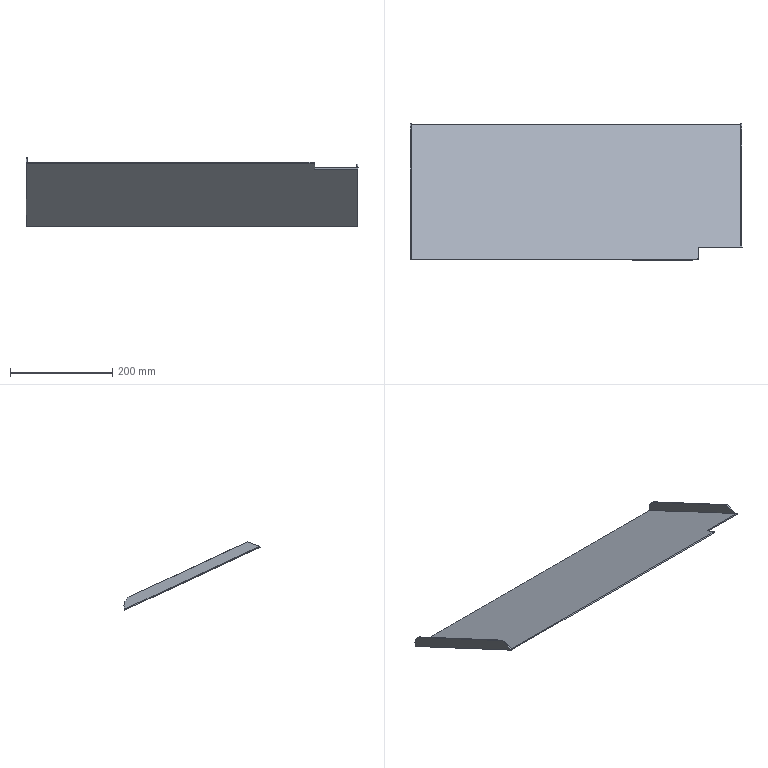Part | NX | features solid 2 | 1 solid | 21 faces | box 650 x 266.54 x 133.86 mm | volume 390473 mm3 | plane 15 | spline 4 | cylinder 2 | commonest cylinder face diameters 40 x2
STEP:
#1=CARTESIAN_POINT('',(363.,820.,-235.638));
#2=VERTEX_POINT('',#1);
#3=CARTESIAN_POINT('',(363.,820.,-233.432));
#4=VERTEX_POINT('',#3);
#5=CARTESIAN_POINT('',(363.,820.,-700.));
#6=DIRECTION('',(0.,0.,-1.));
#7=VECTOR('',#6,1000.);
#8=LINE('',#5,#7);
#9=EDGE_CURVE('',#2,#4,#8,.F.);
#10=ORIENTED_EDGE('',*,*,#9,.F.);
#11=CARTESIAN_POINT('',(280.,820.,-235.638));
#12=VERTEX_POINT('',#11);
#13=CARTESIAN_POINT('',(280.,820.,-235.638));
#14=CARTESIAN_POINT('',(307.667,820.,-235.638));
#15=CARTESIAN_POINT('',(335.333,820.,-235.638));
#16=CARTESIAN_POINT('',(363.,820.,-235.638));
#17=B_SPLINE_CURVE_WITH_KNOTS('',3,(#13,#14,#15,#16),.UNSPECIFIED.,.F.,.F.,(4,4),(0.,0.9765),.UNSPECIFIED.);
#18=EDGE_CURVE('',#12,#2,#17,.T.);
#19=ORIENTED_EDGE('',*,*,#18,.F.);
#20=CARTESIAN_POINT('',(-283.,820.,-235.638));
#21=VERTEX_POINT('',#20);
#22=CARTESIAN_POINT('',(1065.,820.,-235.638));
#23=DIRECTION('',(-1.,0.,0.));
#24=VECTOR('',#23,1000.);
#25=LINE('',#22,#24);
#26=EDGE_CURVE('',#21,#12,#25,.F.);
#27=ORIENTED_EDGE('',*,*,#26,.F.);
#28=CARTESIAN_POINT('',(-283.,820.,-233.432));
#29=VERTEX_POINT('',#28);
#30=CARTESIAN_POINT('',(-283.,820.,-700.));
#31=DIRECTION('',(0.,0.,1.));
#32=VECTOR('',#31,1000.);
#33=LINE('',#30,#32);
#34=EDGE_CURVE('',#29,#21,#33,.F.);
#35=ORIENTED_EDGE('',*,*,#34,.F.);
#36=CARTESIAN_POINT('',(1065.,820.,-233.432));
#37=DIRECTION('',(-1.,0.,0.));
#38=VECTOR('',#37,1000.);
#39=LINE('',#36,#38);
#40=EDGE_CURVE('',#29,#4,#39,.F.);
#41=ORIENTED_EDGE('',*,*,#40,.T.);
#42=EDGE_LOOP('',(#10,#19,#27,#35,#41));
#43=FACE_BOUND('',#42,.T.);
#44=CARTESIAN_POINT('',(1065.,820.,-700.));
#45=DIRECTION('',(0.,-1.,0.));
#46=DIRECTION('',(-1.,0.,0.));
#47=AXIS2_PLACEMENT_3D('',#44,#45,#46);
#48=PLANE('',#47);
#49=ADVANCED_FACE('',(#43),#48,.F.);
#50=CARTESIAN_POINT('',(363.,582.799,-122.823));
#51=VERTEX_POINT('',#50);
#52=CARTESIAN_POINT('',(363.,569.539,-116.64));
#53=DIRECTION('',(0.,-0.9063,0.4226));
#54=VECTOR('',#53,1000.);
#55=LINE('',#52,#54);
#56=EDGE_CURVE('',#4,#51,#55,.T.);
#57=ORIENTED_EDGE('',*,*,#56,.F.);
#58=ORIENTED_EDGE('',*,*,#40,.F.);
#59=CARTESIAN_POINT('',(-283.,556.355,-110.492));
#60=VERTEX_POINT('',#59);
#61=CARTESIAN_POINT('',(-283.,569.539,-116.64));
#62=DIRECTION('',(0.,0.9063,-0.4226));
#63=VECTOR('',#62,1000.);
#64=LINE('',#61,#63);
#65=EDGE_CURVE('',#60,#29,#64,.T.);
#66=ORIENTED_EDGE('',*,*,#65,.F.);
#67=CARTESIAN_POINT('',(280.,557.997,-111.258));
#68=VERTEX_POINT('',#67);
#69=CARTESIAN_POINT('',(-283.,556.355,-110.492));
#70=CARTESIAN_POINT('',(-278.931,556.386,-110.507));
#71=CARTESIAN_POINT('',(-273.683,556.424,-110.524));
#72=CARTESIAN_POINT('',(-269.093,556.45,-110.536));
#73=CARTESIAN_POINT('',(-266.871,556.46,-110.541));
#74=CARTESIAN_POINT('',(-265.734,556.464,-110.543));
#75=CARTESIAN_POINT('',(-264.768,556.467,-110.544));
#76=CARTESIAN_POINT('',(-264.472,556.467,-110.544));
#77=CARTESIAN_POINT('',(-263.335,556.469,-110.545));
#78=CARTESIAN_POINT('',(-260.973,556.47,-110.546));
#79=CARTESIAN_POINT('',(-257.355,556.471,-110.546));
#80=CARTESIAN_POINT('',(-253.755,556.471,-110.546));
#81=CARTESIAN_POINT('',(-251.203,556.471,-110.546));
#82=CARTESIAN_POINT('',(-248.985,556.47,-110.546));
#83=CARTESIAN_POINT('',(-247.518,556.47,-110.546));
#84=CARTESIAN_POINT('',(-246.313,556.47,-110.546));
#85=CARTESIAN_POINT('',(-245.51,556.47,-110.546));
#86=CARTESIAN_POINT('',(-245.,556.47,-110.546));
#87=CARTESIAN_POINT('',(-244.61,556.47,-110.546));
#88=CARTESIAN_POINT('',(-244.577,556.47,-110.546));
#89=CARTESIAN_POINT('',(-244.438,556.47,-110.546));
#90=CARTESIAN_POINT('',(-244.266,556.47,-110.546));
#91=CARTESIAN_POINT('',(-244.029,556.47,-110.546));
#92=CARTESIAN_POINT('',(-243.648,556.47,-110.546));
#93=CARTESIAN_POINT('',(-243.15,556.47,-110.546));
#94=CARTESIAN_POINT('',(-242.522,556.47,-110.546));
#95=CARTESIAN_POINT('',(-241.644,556.47,-110.546));
#96=CARTESIAN_POINT('',(-240.468,556.47,-110.546));
#97=CARTESIAN_POINT('',(-238.932,556.47,-110.546));
#98=CARTESIAN_POINT('',(-237.272,556.47,-110.546));
#99=CARTESIAN_POINT('',(-234.893,556.471,-110.546));
#100=CARTESIAN_POINT('',(-231.608,556.471,-110.546));
#101=CARTESIAN_POINT('',(-227.169,556.472,-110.547));
#102=CARTESIAN_POINT('',(-222.234,556.474,-110.547));
#103=CARTESIAN_POINT('',(-217.705,556.475,-110.548));
#104=CARTESIAN_POINT('',(-213.835,556.477,-110.549));
#105=CARTESIAN_POINT('',(-210.805,556.478,-110.549));
#106=CARTESIAN_POINT('',(-208.187,556.479,-110.55));
#107=CARTESIAN_POINT('',(-206.278,556.479,-110.55));
#108=CARTESIAN_POINT('',(-205.207,556.48,-110.55));
#109=CARTESIAN_POINT('',(-204.295,556.48,-110.55));
#110=CARTESIAN_POINT('',(-203.762,556.48,-110.55));
#111=CARTESIAN_POINT('',(-202.967,556.48,-110.551));
#112=CARTESIAN_POINT('',(-201.617,556.481,-110.551));
#113=CARTESIAN_POINT('',(-199.674,556.482,-110.551));
#114=CARTESIAN_POINT('',(-197.361,556.482,-110.551));
#115=CARTESIAN_POINT('',(-194.288,556.484,-110.552));
#116=CARTESIAN_POINT('',(-190.473,556.485,-110.553));
#117=CARTESIAN_POINT('',(-184.421,556.487,-110.553));
#118=CARTESIAN_POINT('',(-176.957,556.489,-110.554));
#119=CARTESIAN_POINT('',(-168.157,556.491,-110.555));
#120=CARTESIAN_POINT('',(-159.529,556.493,-110.556));
#121=CARTESIAN_POINT('',(-151.02,556.494,-110.557));
#122=CARTESIAN_POINT('',(-144.193,556.495,-110.557));
#123=CARTESIAN_POINT('',(-138.373,556.496,-110.558));
#124=CARTESIAN_POINT('',(-132.608,556.496,-110.558));
#125=CARTESIAN_POINT('',(-122.474,556.497,-110.558));
#126=CARTESIAN_POINT('',(-107.961,556.497,-110.558));
#127=CARTESIAN_POINT('',(-90.461,556.496,-110.558));
#128=CARTESIAN_POINT('',(-67.026,556.492,-110.556));
#129=CARTESIAN_POINT('',(-43.429,556.486,-110.553));
#130=CARTESIAN_POINT('',(-22.654,556.478,-110.549));
#131=CARTESIAN_POINT('',(-10.728,556.473,-110.547));
#132=CARTESIAN_POINT('',(-1.807,556.469,-110.545));
#133=CARTESIAN_POINT('',(7.39,556.464,-110.543));
#134=CARTESIAN_POINT('',(19.483,556.458,-110.54));
#135=CARTESIAN_POINT('',(40.546,556.446,-110.534));
#136=CARTESIAN_POINT('',(64.247,556.429,-110.527));
#137=CARTESIAN_POINT('',(87.609,556.411,-110.518));
#138=CARTESIAN_POINT('',(104.953,556.395,-110.511));
#139=CARTESIAN_POINT('',(119.271,556.382,-110.504));
#140=CARTESIAN_POINT('',(129.2,556.372,-110.5));
#141=CARTESIAN_POINT('',(134.878,556.366,-110.497));
#142=CARTESIAN_POINT('',(139.051,556.361,-110.495));
#143=CARTESIAN_POINT('',(143.632,556.356,-110.493));
#144=CARTESIAN_POINT('',(149.578,556.35,-110.49));
#145=CARTESIAN_POINT('',(160.009,556.338,-110.484));
#146=CARTESIAN_POINT('',(174.758,556.32,-110.476));
#147=CARTESIAN_POINT('',(189.34,556.301,-110.467));
#148=CARTESIAN_POINT('',(200.949,556.285,-110.459));
#149=CARTESIAN_POINT('',(209.492,556.273,-110.454));
#150=CARTESIAN_POINT('',(218.464,556.26,-110.448));
#151=CARTESIAN_POINT('',(227.262,556.247,-110.441));
#152=CARTESIAN_POINT('',(236.065,556.233,-110.435));
#153=CARTESIAN_POINT('',(244.756,556.219,-110.428));
#154=CARTESIAN_POINT('',(252.156,556.206,-110.423));
#155=CARTESIAN_POINT('',(257.28,556.198,-110.419));
#156=CARTESIAN_POINT('',(260.209,556.193,-110.416));
#157=CARTESIAN_POINT('',(262.031,556.189,-110.415));
#158=CARTESIAN_POINT('',(263.502,556.187,-110.414));
#159=CARTESIAN_POINT('',(264.602,556.185,-110.413));
#160=CARTESIAN_POINT('',(265.522,556.183,-110.412));
#161=CARTESIAN_POINT('',(266.158,556.182,-110.411));
#162=CARTESIAN_POINT('',(266.534,556.182,-110.411));
#163=CARTESIAN_POINT('',(266.779,556.181,-110.411));
#164=CARTESIAN_POINT('',(267.335,556.18,-110.411));
#165=CARTESIAN_POINT('',(267.867,556.18,-110.41));
#166=CARTESIAN_POINT('',(268.429,556.179,-110.41));
#167=CARTESIAN_POINT('',(268.765,556.179,-110.41));
#168=CARTESIAN_POINT('',(268.942,556.181,-110.411));
#169=CARTESIAN_POINT('',(268.947,556.18,-110.41));
#170=CARTESIAN_POINT('',(269.298,556.193,-110.417));
#171=CARTESIAN_POINT('',(269.627,556.217,-110.428));
#172=CARTESIAN_POINT('',(270.088,556.271,-110.453));
#173=CARTESIAN_POINT('',(270.202,556.291,-110.462));
#174=CARTESIAN_POINT('',(270.458,556.333,-110.482));
#175=CARTESIAN_POINT('',(270.765,556.386,-110.506));
#176=CARTESIAN_POINT('',(271.258,556.471,-110.546));
#177=CARTESIAN_POINT('',(271.394,556.495,-110.557));
#178=CARTESIAN_POINT('',(271.708,556.55,-110.583));
#179=CARTESIAN_POINT('',(272.066,556.613,-110.612));
#180=CARTESIAN_POINT('',(272.531,556.694,-110.65));
#181=CARTESIAN_POINT('',(273.483,556.86,-110.728));
#182=CARTESIAN_POINT('',(275.728,557.252,-110.91));
#183=CARTESIAN_POINT('',(278.187,557.681,-111.11));
#184=CARTESIAN_POINT('',(280.,557.997,-111.258));
#185=B_SPLINE_CURVE_WITH_KNOTS('',3,(#69,#70,#71,#72,#73,#74,#75,#76,#77,#78,#79,#80,#81,#82,#83,#84,#85,#86,#87,#88,#89,#90,#91,#92,#93,#94,#95,#96,#97,#98,#99,#100,#101,#102,#103,#104,#105,#106,#107,#108,#109,#110,#111,#112,#113,#114,#115,#116,#117,#118,#119,#120,#121,#122,#123,#124,#125,#126,#127,#128,#129,#130,#131,#132,#133,#134,#135,#136,#137,#138,#139,#140,#141,#142,#143,#144,#145,#146,#147,#148,#149,#150,#151,#152,#153,#154,#155,#156,#157,#158,#159,#160,#161,#162,#163,#164,#165,#166,#167,#168,#169,#170,#171,#172,#173,#174,#175,#176,#177,#178,#179,#180,#181,#182,#183,#184),.UNSPECIFIED.,.F.,.F.,(4,1,1,1,1,1,1,1,1,1,1,1,1,1,1,1,1,1,1,1,1,1,1,1,1,1,1,1,1,1,1,1,1,1,1,1,1,1,1,1,1,1,1,1,1,1,1,1,1,1,1,1,1,1,1,1,1,1,1,1,1,1,1,1,1,1,1,1,1,1,1,1,1,1,1,1,1,1,1,1,1,1,1,1,1,1,1,1,1,1,1,1,1,1,1,1,1,1,1,1,1,1,1,1,1,1,1,1,1,1,1,1,1,4),(0.002497,0.01808,0.02588,0.02977,0.03367,0.03562,0.03757,0.04146,0.04925,0.05705,0.06094,0.06484,0.06679,0.06874,0.06971,0.07069,0.07117,0.07142,0.07166,0.07215,0.07263,0.07361,0.07458,0.07653,0.07848,0.08043,0.08432,0.08822,0.09212,0.09601,0.1038,0.1116,0.1194,0.1272,0.1311,0.135,0.1389,0.1408,0.1418,0.1428,0.1437,0.1447,0.1467,0.1506,0.1545,0.1584,0.1661,0.1739,0.1895,0.2051,0.2207,0.2363,0.2519,0.2597,0.2675,0.283,0.3142,0.3454,0.3766,0.4389,0.4701,0.4857,0.5012,0.5168,0.5324,0.5636,0.6259,0.6571,0.6883,0.7195,0.735,0.7428,0.7506,0.7584,0.7662,0.7818,0.813,0.8441,0.8597,0.8753,0.8909,0.9065,0.9221,0.9377,0.9532,0.961,0.9649,0.9688,0.9708,0.9727,0.9747,0.9756,0.9761,0.9766,0.9771,0.9776,0.9786,0.9795,0.98,0.9805,0.981,0.9815,0.9825,0.983,0.9834,0.9839,0.9844,0.9849,0.9854,0.9864,0.9873,0.9883,0.9922,1.),.UNSPECIFIED.);
#186=EDGE_CURVE('',#60,#68,#185,.T.);
#187=ORIENTED_EDGE('',*,*,#186,.T.);
#188=CARTESIAN_POINT('',(280.,580.313,-121.664));
#189=VERTEX_POINT('',#188);
#190=CARTESIAN_POINT('',(280.,569.539,-116.64));
#191=DIRECTION('',(0.,0.9063,-0.4226));
#192=VECTOR('',#191,1000.);
#193=LINE('',#190,#192);
#194=EDGE_CURVE('',#68,#189,#193,.T.);
#195=ORIENTED_EDGE('',*,*,#194,.T.);
#196=CARTESIAN_POINT('',(365.,580.142,-121.584));
#197=VERTEX_POINT('',#196);
#198=CARTESIAN_POINT('',(280.,580.313,-121.664));
#199=CARTESIAN_POINT('',(308.333,580.262,-121.64));
#200=CARTESIAN_POINT('',(336.667,580.205,-121.614));
#201=CARTESIAN_POINT('',(365.,580.142,-121.584));
#202=B_SPLINE_CURVE_WITH_KNOTS('',3,(#198,#199,#200,#201),.UNSPECIFIED.,.F.,.F.,(4,4),(0.,0.085),.UNSPECIFIED.);
#203=EDGE_CURVE('',#189,#197,#202,.T.);
#204=ORIENTED_EDGE('',*,*,#203,.T.);
#205=CARTESIAN_POINT('',(365.,582.799,-122.823));
#206=VERTEX_POINT('',#205);
#207=CARTESIAN_POINT('',(365.,569.539,-116.64));
#208=DIRECTION('',(0.,0.9063,-0.4226));
#209=VECTOR('',#208,1000.);
#210=LINE('',#207,#209);
#211=EDGE_CURVE('',#197,#206,#210,.T.);
#212=ORIENTED_EDGE('',*,*,#211,.T.);
#213=CARTESIAN_POINT('',(-285.,582.799,-122.823));
#214=DIRECTION('',(-1.,0.,0.));
#215=VECTOR('',#214,1000.);
#216=LINE('',#213,#215);
#217=EDGE_CURVE('',#51,#206,#216,.F.);
#218=ORIENTED_EDGE('',*,*,#217,.F.);
#219=EDGE_LOOP('',(#57,#58,#66,#187,#195,#204,#212,#218));
#220=FACE_BOUND('',#219,.T.);
#221=CARTESIAN_POINT('',(-285.,569.539,-116.64));
#222=DIRECTION('',(0.,0.4226,0.9063));
#223=DIRECTION('',(1.,0.,0.));
#224=AXIS2_PLACEMENT_3D('',#221,#222,#223);
#225=PLANE('',#224);
#226=ADVANCED_FACE('',(#220),#225,.T.);
#227=CARTESIAN_POINT('',(-285.,810.326,-209.06));
#228=VERTEX_POINT('',#227);
#229=CARTESIAN_POINT('',(-285.,820.,-235.638));
#230=VERTEX_POINT('',#229);
#231=CARTESIAN_POINT('',(-285.,801.874,-227.186));
#232=DIRECTION('',(1.,0.,0.));
#233=DIRECTION('',(0.,1.,0.));
#234=AXIS2_PLACEMENT_3D('',#231,#232,#233);
#235=CIRCLE('',#234,20.);
#236=EDGE_CURVE('',#228,#230,#235,.F.);
#237=ORIENTED_EDGE('',*,*,#236,.T.);
#238=CARTESIAN_POINT('',(-285.,555.494,-112.297));
#239=VERTEX_POINT('',#238);
#240=CARTESIAN_POINT('',(-285.,568.694,-118.452));
#241=DIRECTION('',(0.,0.9063,-0.4226));
#242=VECTOR('',#241,1000.);
#243=LINE('',#240,#242);
#244=EDGE_CURVE('',#239,#230,#243,.T.);
#245=ORIENTED_EDGE('',*,*,#244,.F.);
#246=CARTESIAN_POINT('',(-285.,556.339,-110.485));
#247=VERTEX_POINT('',#246);
#248=CARTESIAN_POINT('',(-285.,555.494,-112.297));
#249=DIRECTION('',(0.,0.4226,0.9063));
#250=VECTOR('',#249,1000.);
#251=LINE('',#248,#250);
#252=EDGE_CURVE('',#239,#247,#251,.T.);
#253=ORIENTED_EDGE('',*,*,#252,.T.);
#254=CARTESIAN_POINT('',(-285.,580.26,-101.778));
#255=VERTEX_POINT('',#254);
#256=CARTESIAN_POINT('',(-285.,580.26,-101.778));
#257=DIRECTION('',(0.,-0.9397,-0.342));
#258=VECTOR('',#257,1000.);
#259=LINE('',#256,#258);
#260=EDGE_CURVE('',#247,#255,#259,.F.);
#261=ORIENTED_EDGE('',*,*,#260,.T.);
#262=CARTESIAN_POINT('',(-285.,563.946,-94.171));
#263=DIRECTION('',(0.,0.9063,-0.4226));
#264=VECTOR('',#263,1000.);
#265=LINE('',#262,#264);
#266=EDGE_CURVE('',#255,#228,#265,.T.);
#267=ORIENTED_EDGE('',*,*,#266,.T.);
#268=EDGE_LOOP('',(#237,#245,#253,#261,#267));
#269=FACE_BOUND('',#268,.T.);
#270=CARTESIAN_POINT('',(-285.,569.539,-116.64));
#271=DIRECTION('',(-1.,0.,0.));
#272=DIRECTION('',(0.,-1.,0.));
#273=AXIS2_PLACEMENT_3D('',#270,#271,#272);
#274=PLANE('',#273);
#275=ADVANCED_FACE('',(#269),#274,.T.);
#276=ORIENTED_EDGE('',*,*,#186,.F.);
#277=CARTESIAN_POINT('',(-283.,555.502,-112.301));
#278=VERTEX_POINT('',#277);
#279=CARTESIAN_POINT('',(-283.,556.355,-110.492));
#280=DIRECTION('',(0.,-0.4226,-0.9063));
#281=VECTOR('',#280,1000.);
#282=LINE('',#279,#281);
#283=EDGE_CURVE('',#60,#278,#282,.T.);
#284=ORIENTED_EDGE('',*,*,#283,.T.);
#285=CARTESIAN_POINT('',(280.,557.152,-113.07));
#286=VERTEX_POINT('',#285);
#287=CARTESIAN_POINT('',(-283.,555.51,-112.305));
#288=CARTESIAN_POINT('',(-278.931,555.541,-112.319));
#289=CARTESIAN_POINT('',(-273.683,555.578,-112.337));
#290=CARTESIAN_POINT('',(-269.093,555.605,-112.349));
#291=CARTESIAN_POINT('',(-266.871,555.615,-112.354));
#292=CARTESIAN_POINT('',(-265.734,555.619,-112.356));
#293=CARTESIAN_POINT('',(-264.768,555.622,-112.357));
#294=CARTESIAN_POINT('',(-264.472,555.622,-112.357));
#295=CARTESIAN_POINT('',(-263.335,555.623,-112.358));
#296=CARTESIAN_POINT('',(-260.973,555.625,-112.358));
#297=CARTESIAN_POINT('',(-257.355,555.625,-112.359));
#298=CARTESIAN_POINT('',(-253.755,555.625,-112.359));
#299=CARTESIAN_POINT('',(-251.203,555.625,-112.359));
#300=CARTESIAN_POINT('',(-248.985,555.625,-112.358));
#301=CARTESIAN_POINT('',(-247.518,555.625,-112.358));
#302=CARTESIAN_POINT('',(-246.313,555.625,-112.358));
#303=CARTESIAN_POINT('',(-245.51,555.625,-112.358));
#304=CARTESIAN_POINT('',(-245.,555.625,-112.358));
#305=CARTESIAN_POINT('',(-244.61,555.625,-112.358));
#306=CARTESIAN_POINT('',(-244.577,555.625,-112.358));
#307=CARTESIAN_POINT('',(-244.438,555.625,-112.358));
#308=CARTESIAN_POINT('',(-244.266,555.625,-112.358));
#309=CARTESIAN_POINT('',(-244.029,555.625,-112.358));
#310=CARTESIAN_POINT('',(-243.648,555.625,-112.358));
#311=CARTESIAN_POINT('',(-243.15,555.625,-112.358));
#312=CARTESIAN_POINT('',(-242.522,555.625,-112.358));
#313=CARTESIAN_POINT('',(-241.644,555.625,-112.358));
#314=CARTESIAN_POINT('',(-240.468,555.625,-112.358));
#315=CARTESIAN_POINT('',(-238.932,555.625,-112.358));
#316=CARTESIAN_POINT('',(-237.272,555.625,-112.358));
#317=CARTESIAN_POINT('',(-234.893,555.625,-112.359));
#318=CARTESIAN_POINT('',(-231.608,555.626,-112.359));
#319=CARTESIAN_POINT('',(-227.169,555.627,-112.359));
#320=CARTESIAN_POINT('',(-222.234,555.629,-112.36));
#321=CARTESIAN_POINT('',(-217.705,555.63,-112.361));
#322=CARTESIAN_POINT('',(-213.835,555.631,-112.361));
#323=CARTESIAN_POINT('',(-210.805,555.632,-112.362));
#324=CARTESIAN_POINT('',(-208.187,555.633,-112.362));
#325=CARTESIAN_POINT('',(-206.278,555.634,-112.363));
#326=CARTESIAN_POINT('',(-205.207,555.634,-112.363));
#327=CARTESIAN_POINT('',(-204.295,555.635,-112.363));
#328=CARTESIAN_POINT('',(-203.762,555.635,-112.363));
#329=CARTESIAN_POINT('',(-202.967,555.635,-112.363));
#330=CARTESIAN_POINT('',(-201.617,555.636,-112.363));
#331=CARTESIAN_POINT('',(-199.674,555.636,-112.364));
#332=CARTESIAN_POINT('',(-197.361,555.637,-112.364));
#333=CARTESIAN_POINT('',(-194.288,555.638,-112.365));
#334=CARTESIAN_POINT('',(-190.473,555.64,-112.365));
#335=CARTESIAN_POINT('',(-184.421,555.641,-112.366));
#336=CARTESIAN_POINT('',(-176.957,555.644,-112.367));
#337=CARTESIAN_POINT('',(-168.157,555.646,-112.368));
#338=CARTESIAN_POINT('',(-159.529,555.648,-112.369));
#339=CARTESIAN_POINT('',(-151.02,555.649,-112.37));
#340=CARTESIAN_POINT('',(-144.193,555.65,-112.37));
#341=CARTESIAN_POINT('',(-138.373,555.651,-112.37));
#342=CARTESIAN_POINT('',(-132.608,555.651,-112.371));
#343=CARTESIAN_POINT('',(-122.474,555.652,-112.371));
#344=CARTESIAN_POINT('',(-107.961,555.652,-112.371));
#345=CARTESIAN_POINT('',(-90.461,555.65,-112.37));
#346=CARTESIAN_POINT('',(-67.026,555.647,-112.369));
#347=CARTESIAN_POINT('',(-43.429,555.641,-112.366));
#348=CARTESIAN_POINT('',(-22.654,555.633,-112.362));
#349=CARTESIAN_POINT('',(-10.728,555.628,-112.36));
#350=CARTESIAN_POINT('',(-1.807,555.624,-112.358));
#351=CARTESIAN_POINT('',(7.39,555.619,-112.356));
#352=CARTESIAN_POINT('',(19.483,555.613,-112.353));
#353=CARTESIAN_POINT('',(40.546,555.6,-112.347));
#354=CARTESIAN_POINT('',(64.247,555.584,-112.339));
#355=CARTESIAN_POINT('',(87.609,555.565,-112.331));
#356=CARTESIAN_POINT('',(104.953,555.55,-112.323));
#357=CARTESIAN_POINT('',(119.271,555.536,-112.317));
#358=CARTESIAN_POINT('',(129.2,555.526,-112.312));
#359=CARTESIAN_POINT('',(134.878,555.52,-112.31));
#360=CARTESIAN_POINT('',(139.051,555.516,-112.308));
#361=CARTESIAN_POINT('',(143.632,555.511,-112.305));
#362=CARTESIAN_POINT('',(149.578,555.504,-112.302));
#363=CARTESIAN_POINT('',(160.009,555.492,-112.297));
#364=CARTESIAN_POINT('',(174.758,555.475,-112.288));
#365=CARTESIAN_POINT('',(189.34,555.456,-112.279));
#366=CARTESIAN_POINT('',(200.949,555.44,-112.272));
#367=CARTESIAN_POINT('',(209.492,555.428,-112.266));
#368=CARTESIAN_POINT('',(218.464,555.415,-112.26));
#369=CARTESIAN_POINT('',(227.262,555.401,-112.254));
#370=CARTESIAN_POINT('',(236.065,555.388,-112.248));
#371=CARTESIAN_POINT('',(244.756,555.374,-112.241));
#372=CARTESIAN_POINT('',(252.156,555.361,-112.235));
#373=CARTESIAN_POINT('',(257.28,555.352,-112.231));
#374=CARTESIAN_POINT('',(260.209,555.347,-112.229));
#375=CARTESIAN_POINT('',(262.031,555.344,-112.227));
#376=CARTESIAN_POINT('',(263.502,555.342,-112.226));
#377=CARTESIAN_POINT('',(264.602,555.34,-112.225));
#378=CARTESIAN_POINT('',(265.522,555.338,-112.225));
#379=CARTESIAN_POINT('',(266.158,555.337,-112.224));
#380=CARTESIAN_POINT('',(266.534,555.336,-112.224));
#381=CARTESIAN_POINT('',(266.779,555.336,-112.224));
#382=CARTESIAN_POINT('',(267.335,555.335,-112.223));
#383=CARTESIAN_POINT('',(267.867,555.334,-112.223));
#384=CARTESIAN_POINT('',(268.429,555.334,-112.223));
#385=CARTESIAN_POINT('',(268.765,555.334,-112.223));
#386=CARTESIAN_POINT('',(268.942,555.336,-112.224));
#387=CARTESIAN_POINT('',(268.947,555.334,-112.223));
#388=CARTESIAN_POINT('',(269.298,555.348,-112.229));
#389=CARTESIAN_POINT('',(269.627,555.372,-112.24));
#390=CARTESIAN_POINT('',(270.088,555.426,-112.266));
#391=CARTESIAN_POINT('',(270.202,555.446,-112.275));
#392=CARTESIAN_POINT('',(270.458,555.488,-112.294));
#393=CARTESIAN_POINT('',(270.765,555.54,-112.319));
#394=CARTESIAN_POINT('',(271.258,555.626,-112.359));
#395=CARTESIAN_POINT('',(271.394,555.65,-112.37));
#396=CARTESIAN_POINT('',(271.708,555.705,-112.396));
#397=CARTESIAN_POINT('',(272.066,555.767,-112.425));
#398=CARTESIAN_POINT('',(272.531,555.848,-112.463));
#399=CARTESIAN_POINT('',(273.483,556.015,-112.54));
#400=CARTESIAN_POINT('',(275.728,556.407,-112.723));
#401=CARTESIAN_POINT('',(278.187,556.836,-112.923));
#402=CARTESIAN_POINT('',(280.,557.152,-113.07));
#403=B_SPLINE_CURVE_WITH_KNOTS('',3,(#287,#288,#289,#290,#291,#292,#293,#294,#295,#296,#297,#298,#299,#300,#301,#302,#303,#304,#305,#306,#307,#308,#309,#310,#311,#312,#313,#314,#315,#316,#317,#318,#319,#320,#321,#322,#323,#324,#325,#326,#327,#328,#329,#330,#331,#332,#333,#334,#335,#336,#337,#338,#339,#340,#341,#342,#343,#344,#345,#346,#347,#348,#349,#350,#351,#352,#353,#354,#355,#356,#357,#358,#359,#360,#361,#362,#363,#364,#365,#366,#367,#368,#369,#370,#371,#372,#373,#374,#375,#376,#377,#378,#379,#380,#381,#382,#383,#384,#385,#386,#387,#388,#389,#390,#391,#392,#393,#394,#395,#396,#397,#398,#399,#400,#401,#402),.UNSPECIFIED.,.F.,.F.,(4,1,1,1,1,1,1,1,1,1,1,1,1,1,1,1,1,1,1,1,1,1,1,1,1,1,1,1,1,1,1,1,1,1,1,1,1,1,1,1,1,1,1,1,1,1,1,1,1,1,1,1,1,1,1,1,1,1,1,1,1,1,1,1,1,1,1,1,1,1,1,1,1,1,1,1,1,1,1,1,1,1,1,1,1,1,1,1,1,1,1,1,1,1,1,1,1,1,1,1,1,1,1,1,1,1,1,1,1,1,1,1,1,4),(0.002497,0.01808,0.02588,0.02977,0.03367,0.03562,0.03757,0.04146,0.04925,0.05705,0.06094,0.06484,0.06679,0.06874,0.06971,0.07069,0.07117,0.07142,0.07166,0.07215,0.07263,0.07361,0.07458,0.07653,0.07848,0.08043,0.08432,0.08822,0.09212,0.09601,0.1038,0.1116,0.1194,0.1272,0.1311,0.135,0.1389,0.1408,0.1418,0.1428,0.1437,0.1447,0.1467,0.1506,0.1545,0.1584,0.1661,0.1739,0.1895,0.2051,0.2207,0.2363,0.2519,0.2597,0.2675,0.283,0.3142,0.3454,0.3766,0.4389,0.4701,0.4857,0.5012,0.5168,0.5324,0.5636,0.6259,0.6571,0.6883,0.7195,0.735,0.7428,0.7506,0.7584,0.7662,0.7818,0.813,0.8441,0.8597,0.8753,0.8909,0.9065,0.9221,0.9377,0.9532,0.961,0.9649,0.9688,0.9708,0.9727,0.9747,0.9756,0.9761,0.9766,0.9771,0.9776,0.9786,0.9795,0.98,0.9805,0.981,0.9815,0.9825,0.983,0.9834,0.9839,0.9844,0.9849,0.9854,0.9864,0.9873,0.9883,0.9922,1.),.UNSPECIFIED.);
#404=EDGE_CURVE('',#278,#286,#403,.T.);
#405=ORIENTED_EDGE('',*,*,#404,.T.);
#406=CARTESIAN_POINT('',(280.,557.997,-111.258));
#407=CARTESIAN_POINT('',(280.,557.716,-111.862));
#408=CARTESIAN_POINT('',(280.,557.434,-112.466));
#409=CARTESIAN_POINT('',(280.,557.152,-113.07));
#410=B_SPLINE_CURVE_WITH_KNOTS('',3,(#406,#407,#408,#409),.UNSPECIFIED.,.F.,.F.,(4,4),(0.,1.),.UNSPECIFIED.);
#411=EDGE_CURVE('',#68,#286,#410,.T.);
#412=ORIENTED_EDGE('',*,*,#411,.F.);
#413=EDGE_LOOP('',(#276,#284,#405,#412));
#414=FACE_BOUND('',#413,.T.);
#415=CARTESIAN_POINT('',(-285.,556.339,-110.485));
#416=CARTESIAN_POINT('',(-285.,555.494,-112.297));
#417=CARTESIAN_POINT('',(-280.736,556.373,-110.5));
#418=CARTESIAN_POINT('',(-280.736,555.528,-112.313));
#419=CARTESIAN_POINT('',(-275.207,556.413,-110.519));
#420=CARTESIAN_POINT('',(-275.207,555.568,-112.332));
#421=CARTESIAN_POINT('',(-270.272,556.444,-110.533));
#422=CARTESIAN_POINT('',(-270.272,555.598,-112.346));
#423=CARTESIAN_POINT('',(-267.89,556.456,-110.539));
#424=CARTESIAN_POINT('',(-267.89,555.611,-112.352));
#425=CARTESIAN_POINT('',(-266.572,556.461,-110.542));
#426=CARTESIAN_POINT('',(-266.572,555.616,-112.354));
#427=CARTESIAN_POINT('',(-265.648,556.465,-110.543));
#428=CARTESIAN_POINT('',(-265.648,555.619,-112.356));
#429=CARTESIAN_POINT('',(-265.067,556.466,-110.544));
#430=CARTESIAN_POINT('',(-265.067,555.621,-112.356));
#431=CARTESIAN_POINT('',(-264.741,556.467,-110.544));
#432=CARTESIAN_POINT('',(-264.741,555.622,-112.357));
#433=CARTESIAN_POINT('',(-264.562,556.467,-110.544));
#434=CARTESIAN_POINT('',(-264.562,555.622,-112.357));
#435=CARTESIAN_POINT('',(-264.088,556.468,-110.545));
#436=CARTESIAN_POINT('',(-264.088,555.623,-112.357));
#437=CARTESIAN_POINT('',(-263.227,556.469,-110.545));
#438=CARTESIAN_POINT('',(-263.227,555.623,-112.358));
#439=CARTESIAN_POINT('',(-261.346,556.47,-110.546));
#440=CARTESIAN_POINT('',(-261.346,555.624,-112.358));
#441=CARTESIAN_POINT('',(-258.749,556.47,-110.546));
#442=CARTESIAN_POINT('',(-258.749,555.625,-112.358));
#443=CARTESIAN_POINT('',(-255.427,556.471,-110.546));
#444=CARTESIAN_POINT('',(-255.427,555.625,-112.359));
#445=CARTESIAN_POINT('',(-253.051,556.471,-110.546));
#446=CARTESIAN_POINT('',(-253.051,555.625,-112.359));
#447=CARTESIAN_POINT('',(-250.969,556.471,-110.546));
#448=CARTESIAN_POINT('',(-250.969,555.625,-112.359));
#449=CARTESIAN_POINT('',(-249.318,556.47,-110.546));
#450=CARTESIAN_POINT('',(-249.318,555.625,-112.358));
#451=CARTESIAN_POINT('',(-247.866,556.47,-110.546));
#452=CARTESIAN_POINT('',(-247.866,555.625,-112.358));
#453=CARTESIAN_POINT('',(-246.662,556.47,-110.546));
#454=CARTESIAN_POINT('',(-246.662,555.625,-112.358));
#455=CARTESIAN_POINT('',(-245.882,556.47,-110.546));
#456=CARTESIAN_POINT('',(-245.882,555.625,-112.358));
#457=CARTESIAN_POINT('',(-245.268,556.47,-110.546));
#458=CARTESIAN_POINT('',(-245.268,555.625,-112.358));
#459=CARTESIAN_POINT('',(-244.831,556.47,-110.546));
#460=CARTESIAN_POINT('',(-244.831,555.625,-112.358));
#461=CARTESIAN_POINT('',(-244.59,556.47,-110.546));
#462=CARTESIAN_POINT('',(-244.59,555.625,-112.358));
#463=CARTESIAN_POINT('',(-244.538,556.47,-110.546));
#464=CARTESIAN_POINT('',(-244.538,555.625,-112.358));
#465=CARTESIAN_POINT('',(-244.357,556.47,-110.546));
#466=CARTESIAN_POINT('',(-244.357,555.625,-112.358));
#467=CARTESIAN_POINT('',(-244.139,556.47,-110.546));
#468=CARTESIAN_POINT('',(-244.139,555.625,-112.358));
#469=CARTESIAN_POINT('',(-243.754,556.47,-110.546));
#470=CARTESIAN_POINT('',(-243.754,555.625,-112.358));
#471=CARTESIAN_POINT('',(-243.263,556.47,-110.546));
#472=CARTESIAN_POINT('',(-243.263,555.625,-112.358));
#473=CARTESIAN_POINT('',(-242.43,556.47,-110.546));
#474=CARTESIAN_POINT('',(-242.43,555.624,-112.358));
#475=CARTESIAN_POINT('',(-241.313,556.47,-110.546));
#476=CARTESIAN_POINT('',(-241.313,555.625,-112.358));
#477=CARTESIAN_POINT('',(-239.358,556.47,-110.546));
#478=CARTESIAN_POINT('',(-239.358,555.625,-112.358));
#479=CARTESIAN_POINT('',(-236.602,556.47,-110.546));
#480=CARTESIAN_POINT('',(-236.602,555.625,-112.358));
#481=CARTESIAN_POINT('',(-232.794,556.471,-110.546));
#482=CARTESIAN_POINT('',(-232.794,555.626,-112.359));
#483=CARTESIAN_POINT('',(-228.487,556.472,-110.547));
#484=CARTESIAN_POINT('',(-228.487,555.627,-112.359));
#485=CARTESIAN_POINT('',(-223.68,556.473,-110.547));
#486=CARTESIAN_POINT('',(-223.68,555.628,-112.36));
#487=CARTESIAN_POINT('',(-219.258,556.475,-110.548));
#488=CARTESIAN_POINT('',(-219.258,555.629,-112.36));
#489=CARTESIAN_POINT('',(-215.471,556.476,-110.548));
#490=CARTESIAN_POINT('',(-215.471,555.631,-112.361));
#491=CARTESIAN_POINT('',(-212.504,556.477,-110.549));
#492=CARTESIAN_POINT('',(-212.504,555.632,-112.362));
#493=CARTESIAN_POINT('',(-209.417,556.478,-110.549));
#494=CARTESIAN_POINT('',(-209.417,555.633,-112.362));
#495=CARTESIAN_POINT('',(-206.994,556.479,-110.55));
#496=CARTESIAN_POINT('',(-206.994,555.634,-112.362));
#497=CARTESIAN_POINT('',(-205.362,556.48,-110.55));
#498=CARTESIAN_POINT('',(-205.362,555.634,-112.363));
#499=CARTESIAN_POINT('',(-204.642,556.48,-110.55));
#500=CARTESIAN_POINT('',(-204.642,555.635,-112.363));
#501=CARTESIAN_POINT('',(-204.141,556.48,-110.55));
#502=CARTESIAN_POINT('',(-204.141,555.635,-112.363));
#503=CARTESIAN_POINT('',(-203.778,556.48,-110.55));
#504=CARTESIAN_POINT('',(-203.778,555.635,-112.363));
#505=CARTESIAN_POINT('',(-203.078,556.48,-110.551));
#506=CARTESIAN_POINT('',(-203.078,555.635,-112.363));
#507=CARTESIAN_POINT('',(-202.113,556.481,-110.551));
#508=CARTESIAN_POINT('',(-202.113,555.636,-112.363));
#509=CARTESIAN_POINT('',(-200.554,556.481,-110.551));
#510=CARTESIAN_POINT('',(-200.554,555.636,-112.364));
#511=CARTESIAN_POINT('',(-198.617,556.482,-110.551));
#512=CARTESIAN_POINT('',(-198.617,555.637,-112.364));
#513=CARTESIAN_POINT('',(-193.985,556.484,-110.552));
#514=CARTESIAN_POINT('',(-193.985,555.638,-112.365));
#515=CARTESIAN_POINT('',(-187.114,556.486,-110.553));
#516=CARTESIAN_POINT('',(-187.114,555.641,-112.366));
#517=CARTESIAN_POINT('',(-178.113,556.489,-110.554));
#518=CARTESIAN_POINT('',(-178.113,555.643,-112.367));
#519=CARTESIAN_POINT('',(-169.274,556.491,-110.555));
#520=CARTESIAN_POINT('',(-169.274,555.646,-112.368));
#521=CARTESIAN_POINT('',(-160.591,556.493,-110.556));
#522=CARTESIAN_POINT('',(-160.591,555.647,-112.369));
#523=CARTESIAN_POINT('',(-153.506,556.494,-110.557));
#524=CARTESIAN_POINT('',(-153.506,555.649,-112.369));
#525=CARTESIAN_POINT('',(-147.883,556.495,-110.557));
#526=CARTESIAN_POINT('',(-147.883,555.65,-112.37));
#527=CARTESIAN_POINT('',(-143.801,556.495,-110.557));
#528=CARTESIAN_POINT('',(-143.801,555.65,-112.37));
#529=CARTESIAN_POINT('',(-139.397,556.496,-110.558));
#530=CARTESIAN_POINT('',(-139.397,555.651,-112.37));
#531=CARTESIAN_POINT('',(-133.628,556.496,-110.558));
#532=CARTESIAN_POINT('',(-133.628,555.651,-112.371));
#533=CARTESIAN_POINT('',(-123.465,556.497,-110.558));
#534=CARTESIAN_POINT('',(-123.465,555.652,-112.371));
#535=CARTESIAN_POINT('',(-108.923,556.497,-110.558));
#536=CARTESIAN_POINT('',(-108.923,555.652,-112.371));
#537=CARTESIAN_POINT('',(-91.383,556.496,-110.558));
#538=CARTESIAN_POINT('',(-91.383,555.65,-112.37));
#539=CARTESIAN_POINT('',(-67.895,556.492,-110.556));
#540=CARTESIAN_POINT('',(-67.895,555.647,-112.369));
#541=CARTESIAN_POINT('',(-44.241,556.486,-110.553));
#542=CARTESIAN_POINT('',(-44.241,555.641,-112.366));
#543=CARTESIAN_POINT('',(-23.424,556.478,-110.55));
#544=CARTESIAN_POINT('',(-23.424,555.633,-112.362));
#545=CARTESIAN_POINT('',(-11.461,556.473,-110.547));
#546=CARTESIAN_POINT('',(-11.461,555.628,-112.36));
#547=CARTESIAN_POINT('',(-2.548,556.469,-110.545));
#548=CARTESIAN_POINT('',(-2.548,555.624,-112.358));
#549=CARTESIAN_POINT('',(6.685,556.465,-110.543));
#550=CARTESIAN_POINT('',(6.685,555.62,-112.356));
#551=CARTESIAN_POINT('',(18.81,556.458,-110.54));
#552=CARTESIAN_POINT('',(18.81,555.613,-112.353));
#553=CARTESIAN_POINT('',(39.935,556.446,-110.535));
#554=CARTESIAN_POINT('',(39.935,555.601,-112.347));
#555=CARTESIAN_POINT('',(63.702,556.43,-110.527));
#556=CARTESIAN_POINT('',(63.702,555.584,-112.339));
#557=CARTESIAN_POINT('',(87.13,556.411,-110.518));
#558=CARTESIAN_POINT('',(87.13,555.566,-112.331));
#559=CARTESIAN_POINT('',(104.52,556.396,-110.511));
#560=CARTESIAN_POINT('',(104.52,555.55,-112.324));
#561=CARTESIAN_POINT('',(118.881,556.382,-110.505));
#562=CARTESIAN_POINT('',(118.881,555.537,-112.317));
#563=CARTESIAN_POINT('',(128.83,556.372,-110.5));
#564=CARTESIAN_POINT('',(128.83,555.527,-112.313));
#565=CARTESIAN_POINT('',(134.536,556.366,-110.497));
#566=CARTESIAN_POINT('',(134.536,555.521,-112.31));
#567=CARTESIAN_POINT('',(138.682,556.362,-110.495));
#568=CARTESIAN_POINT('',(138.682,555.516,-112.308));
#569=CARTESIAN_POINT('',(143.286,556.357,-110.493));
#570=CARTESIAN_POINT('',(143.286,555.511,-112.305));
#571=CARTESIAN_POINT('',(149.245,556.35,-110.49));
#572=CARTESIAN_POINT('',(149.245,555.505,-112.302));
#573=CARTESIAN_POINT('',(159.706,556.338,-110.484));
#574=CARTESIAN_POINT('',(159.706,555.493,-112.297));
#575=CARTESIAN_POINT('',(174.494,556.32,-110.476));
#576=CARTESIAN_POINT('',(174.494,555.475,-112.288));
#577=CARTESIAN_POINT('',(189.114,556.301,-110.467));
#578=CARTESIAN_POINT('',(189.114,555.456,-112.28));
#579=CARTESIAN_POINT('',(200.756,556.285,-110.46));
#580=CARTESIAN_POINT('',(200.756,555.44,-112.272));
#581=CARTESIAN_POINT('',(209.311,556.273,-110.454));
#582=CARTESIAN_POINT('',(209.311,555.428,-112.267));
#583=CARTESIAN_POINT('',(218.31,556.26,-110.448));
#584=CARTESIAN_POINT('',(218.31,555.415,-112.26));
#585=CARTESIAN_POINT('',(227.129,556.247,-110.442));
#586=CARTESIAN_POINT('',(227.129,555.401,-112.254));
#587=CARTESIAN_POINT('',(235.956,556.233,-110.435));
#588=CARTESIAN_POINT('',(235.956,555.388,-112.248));
#589=CARTESIAN_POINT('',(244.666,556.219,-110.429));
#590=CARTESIAN_POINT('',(244.666,555.374,-112.241));
#591=CARTESIAN_POINT('',(252.086,556.207,-110.423));
#592=CARTESIAN_POINT('',(252.086,555.361,-112.235));
#593=CARTESIAN_POINT('',(257.223,556.198,-110.419));
#594=CARTESIAN_POINT('',(257.223,555.353,-112.231));
#595=CARTESIAN_POINT('',(260.16,556.193,-110.416));
#596=CARTESIAN_POINT('',(260.16,555.347,-112.229));
#597=CARTESIAN_POINT('',(261.985,556.19,-110.415));
#598=CARTESIAN_POINT('',(261.985,555.344,-112.227));
#599=CARTESIAN_POINT('',(263.461,556.187,-110.414));
#600=CARTESIAN_POINT('',(263.461,555.342,-112.226));
#601=CARTESIAN_POINT('',(264.561,556.185,-110.413));
#602=CARTESIAN_POINT('',(264.561,555.34,-112.225));
#603=CARTESIAN_POINT('',(265.49,556.183,-110.412));
#604=CARTESIAN_POINT('',(265.49,555.338,-112.225));
#605=CARTESIAN_POINT('',(266.117,556.182,-110.411));
#606=CARTESIAN_POINT('',(266.117,555.337,-112.224));
#607=CARTESIAN_POINT('',(266.511,556.182,-110.411));
#608=CARTESIAN_POINT('',(266.511,555.336,-112.224));
#609=CARTESIAN_POINT('',(266.705,556.181,-110.411));
#610=CARTESIAN_POINT('',(266.705,555.336,-112.224));
#611=CARTESIAN_POINT('',(267.285,556.18,-110.411));
#612=CARTESIAN_POINT('',(267.285,555.335,-112.223));
#613=CARTESIAN_POINT('',(267.822,556.18,-110.41));
#614=CARTESIAN_POINT('',(267.822,555.334,-112.223));
#615=CARTESIAN_POINT('',(268.402,556.179,-110.41));
#616=CARTESIAN_POINT('',(268.402,555.334,-112.223));
#617=CARTESIAN_POINT('',(268.742,556.179,-110.41));
#618=CARTESIAN_POINT('',(268.742,555.334,-112.223));
#619=CARTESIAN_POINT('',(268.941,556.181,-110.411));
#620=CARTESIAN_POINT('',(268.941,555.336,-112.224));
#621=CARTESIAN_POINT('',(268.912,556.179,-110.41));
#622=CARTESIAN_POINT('',(268.912,555.334,-112.222));
#623=CARTESIAN_POINT('',(269.27,556.191,-110.416));
#624=CARTESIAN_POINT('',(269.27,555.346,-112.228));
#625=CARTESIAN_POINT('',(269.528,556.211,-110.425));
#626=CARTESIAN_POINT('',(269.528,555.365,-112.237));
#627=CARTESIAN_POINT('',(269.794,556.235,-110.436));
#628=CARTESIAN_POINT('',(269.794,555.39,-112.249));
#629=CARTESIAN_POINT('',(270.126,556.277,-110.456));
#630=CARTESIAN_POINT('',(270.126,555.432,-112.268));
#631=CARTESIAN_POINT('',(270.181,556.287,-110.461));
#632=CARTESIAN_POINT('',(270.181,555.442,-112.273));
#633=CARTESIAN_POINT('',(270.438,556.329,-110.48));
#634=CARTESIAN_POINT('',(270.438,555.484,-112.293));
#635=CARTESIAN_POINT('',(270.727,556.379,-110.503));
#636=CARTESIAN_POINT('',(270.727,555.534,-112.316));
#637=CARTESIAN_POINT('',(271.247,556.469,-110.545));
#638=CARTESIAN_POINT('',(271.247,555.624,-112.358));
#639=CARTESIAN_POINT('',(271.376,556.492,-110.556));
#640=CARTESIAN_POINT('',(271.376,555.647,-112.369));
#641=CARTESIAN_POINT('',(271.692,556.547,-110.582));
#642=CARTESIAN_POINT('',(271.692,555.702,-112.394));
#643=CARTESIAN_POINT('',(272.05,556.61,-110.611));
#644=CARTESIAN_POINT('',(272.05,555.764,-112.423));
#645=CARTESIAN_POINT('',(272.515,556.691,-110.649));
#646=CARTESIAN_POINT('',(272.515,555.846,-112.461));
#647=CARTESIAN_POINT('',(273.469,556.858,-110.726));
#648=CARTESIAN_POINT('',(273.469,556.012,-112.539));
#649=CARTESIAN_POINT('',(275.718,557.25,-110.909));
#650=CARTESIAN_POINT('',(275.718,556.405,-112.722));
#651=CARTESIAN_POINT('',(278.182,557.68,-111.11));
#652=CARTESIAN_POINT('',(278.182,556.835,-112.923));
#653=CARTESIAN_POINT('',(280.,557.997,-111.258));
#654=CARTESIAN_POINT('',(280.,557.152,-113.07));
#655=B_SPLINE_SURFACE_WITH_KNOTS('',3,1,((#415,#416),(#417,#418),(#419,#420),(#421,#422),(#423,#424),(#425,#426),(#427,#428),(#429,#430),(#431,#432),(#433,#434),(#435,#436),(#437,#438),(#439,#440),(#441,#442),(#443,#444),(#445,#446),(#447,#448),(#449,#450),(#451,#452),(#453,#454),(#455,#456),(#457,#458),(#459,#460),(#461,#462),(#463,#464),(#465,#466),(#467,#468),(#469,#470),(#471,#472),(#473,#474),(#475,#476),(#477,#478),(#479,#480),(#481,#482),(#483,#484),(#485,#486),(#487,#488),(#489,#490),(#491,#492),(#493,#494),(#495,#496),(#497,#498),(#499,#500),(#501,#502),(#503,#504),(#505,#506),(#507,#508),(#509,#510),(#511,#512),(#513,#514),(#515,#516),(#517,#518),(#519,#520),(#521,#522),(#523,#524),(#525,#526),(#527,#528),(#529,#530),(#531,#532),(#533,#534),(#535,#536),(#537,#538),(#539,#540),(#541,#542),(#543,#544),(#545,#546),(#547,#548),(#549,#550),(#551,#552),(#553,#554),(#555,#556),(#557,#558),(#559,#560),(#561,#562),(#563,#564),(#565,#566),(#567,#568),(#569,#570),(#571,#572),(#573,#574),(#575,#576),(#577,#578),(#579,#580),(#581,#582),(#583,#584),(#585,#586),(#587,#588),(#589,#590),(#591,#592),(#593,#594),(#595,#596),(#597,#598),(#599,#600),(#601,#602),(#603,#604),(#605,#606),(#607,#608),(#609,#610),(#611,#612),(#613,#614),(#615,#616),(#617,#618),(#619,#620),(#621,#622),(#623,#624),(#625,#626),(#627,#628),(#629,#630),(#631,#632),(#633,#634),(#635,#636),(#637,#638),(#639,#640),(#641,#642),(#643,#644),(#645,#646),(#647,#648),(#649,#650),(#651,#652),(#653,#654)),.SURF_OF_LINEAR_EXTRUSION.,.F.,.F.,.F.,(4,1,1,1,1,1,1,1,1,1,1,1,1,1,1,1,1,1,1,1,1,1,1,1,1,1,1,1,1,1,1,1,1,1,1,1,1,1,1,1,1,1,1,1,1,1,1,1,1,1,1,1,1,1,1,1,1,1,1,1,1,1,1,1,1,1,1,1,1,1,1,1,1,1,1,1,1,1,1,1,1,1,1,1,1,1,1,1,1,1,1,1,1,1,1,1,1,1,1,1,1,1,1,1,1,1,1,1,1,1,1,1,1,1,1,1,1,4),(2,2),(0.,0.01562,0.02344,0.02734,0.03125,0.0332,0.03516,0.03613,0.03711,0.03906,0.04297,0.04688,0.05469,0.05859,0.0625,0.06445,0.06641,0.06836,0.06934,0.07031,0.0708,0.07129,0.07153,0.07178,0.07227,0.07324,0.07422,0.07617,0.07812,0.08203,0.08594,0.09375,0.1016,0.1094,0.1172,0.125,0.1289,0.1328,0.1367,0.1406,0.1416,0.1426,0.1431,0.1436,0.1445,0.1465,0.1484,0.1523,0.1562,0.1719,0.1875,0.2031,0.2188,0.2344,0.2422,0.25,0.2578,0.2656,0.2812,0.3125,0.3438,0.375,0.4375,0.4688,0.4844,0.5,0.5156,0.5312,0.5625,0.625,0.6562,0.6875,0.7188,0.7344,0.7422,0.75,0.7578,0.7656,0.7812,0.8125,0.8438,0.8594,0.875,0.8906,0.9062,0.9219,0.9375,0.9531,0.9609,0.9648,0.9688,0.9707,0.9727,0.9746,0.9756,0.9761,0.9766,0.9771,0.9775,0.9785,0.9795,0.98,0.9805,0.981,0.9814,0.9819,0.9824,0.9829,0.9834,0.9839,0.9844,0.9849,0.9854,0.9863,0.9873,0.9883,0.9922,1.),(0.,1.),.UNSPECIFIED.);
#656=ADVANCED_FACE('',(#414),#655,.F.);
#657=CARTESIAN_POINT('',(280.,580.313,-123.87));
#658=VERTEX_POINT('',#657);
#659=CARTESIAN_POINT('',(280.,557.152,-113.07));
#660=CARTESIAN_POINT('',(280.,564.872,-116.67));
#661=CARTESIAN_POINT('',(280.,572.592,-120.27));
#662=CARTESIAN_POINT('',(280.,580.313,-123.87));
#663=B_SPLINE_CURVE_WITH_KNOTS('',3,(#659,#660,#661,#662),.UNSPECIFIED.,.F.,.F.,(4,4),(0.,0.1515),.UNSPECIFIED.);
#664=EDGE_CURVE('',#286,#658,#663,.T.);
#665=ORIENTED_EDGE('',*,*,#664,.T.);
#666=CARTESIAN_POINT('',(280.,580.313,-114.327));
#667=DIRECTION('',(0.,0.,-1.));
#668=VECTOR('',#667,1000.);
#669=LINE('',#666,#668);
#670=EDGE_CURVE('',#658,#189,#669,.F.);
#671=ORIENTED_EDGE('',*,*,#670,.T.);
#672=ORIENTED_EDGE('',*,*,#194,.F.);
#673=ORIENTED_EDGE('',*,*,#411,.T.);
#674=EDGE_LOOP('',(#665,#671,#672,#673));
#675=FACE_BOUND('',#674,.T.);
#676=CARTESIAN_POINT('',(280.,569.539,-116.64));
#677=DIRECTION('',(-1.,0.,0.));
#678=DIRECTION('',(0.,0.,1.));
#679=AXIS2_PLACEMENT_3D('',#676,#677,#678);
#680=PLANE('',#679);
#681=ADVANCED_FACE('',(#675),#680,.F.);
#682=ORIENTED_EDGE('',*,*,#18,.T.);
#683=CARTESIAN_POINT('',(365.,820.,-235.638));
#684=VERTEX_POINT('',#683);
#685=CARTESIAN_POINT('',(365.,820.,-235.638));
#686=CARTESIAN_POINT('',(364.333,820.,-235.638));
#687=CARTESIAN_POINT('',(363.667,820.,-235.638));
#688=CARTESIAN_POINT('',(363.,820.,-235.638));
#689=B_SPLINE_CURVE_WITH_KNOTS('',3,(#685,#686,#687,#688),.UNSPECIFIED.,.F.,.F.,(4,4),(0.,0.02353),.UNSPECIFIED.);
#690=EDGE_CURVE('',#684,#2,#689,.T.);
#691=ORIENTED_EDGE('',*,*,#690,.F.);
#692=CARTESIAN_POINT('',(365.,580.142,-123.791));
#693=VERTEX_POINT('',#692);
#694=CARTESIAN_POINT('',(365.,580.142,-123.791));
#695=CARTESIAN_POINT('',(365.,660.094,-161.073));
#696=CARTESIAN_POINT('',(365.,740.047,-198.356));
#697=CARTESIAN_POINT('',(365.,820.,-235.638));
#698=B_SPLINE_CURVE_WITH_KNOTS('',3,(#694,#695,#696,#697),.UNSPECIFIED.,.F.,.F.,(4,4),(0.08746,1.),.UNSPECIFIED.);
#699=EDGE_CURVE('',#693,#684,#698,.T.);
#700=ORIENTED_EDGE('',*,*,#699,.F.);
#701=CARTESIAN_POINT('',(363.,580.146,-123.793));
#702=VERTEX_POINT('',#701);
#703=CARTESIAN_POINT('',(363.,580.146,-123.793));
#704=CARTESIAN_POINT('',(363.667,580.145,-123.792));
#705=CARTESIAN_POINT('',(364.333,580.143,-123.791));
#706=CARTESIAN_POINT('',(365.,580.142,-123.791));
#707=B_SPLINE_CURVE_WITH_KNOTS('',3,(#703,#704,#705,#706),.UNSPECIFIED.,.F.,.F.,(4,4),(0.085,0.087),.UNSPECIFIED.);
#708=EDGE_CURVE('',#702,#693,#707,.T.);
#709=ORIENTED_EDGE('',*,*,#708,.F.);
#710=CARTESIAN_POINT('',(280.,580.313,-123.87));
#711=CARTESIAN_POINT('',(307.667,580.263,-123.847));
#712=CARTESIAN_POINT('',(335.333,580.208,-123.822));
#713=CARTESIAN_POINT('',(363.,580.146,-123.793));
#714=B_SPLINE_CURVE_WITH_KNOTS('',3,(#710,#711,#712,#713),.UNSPECIFIED.,.F.,.F.,(4,4),(0.002,0.085),.UNSPECIFIED.);
#715=EDGE_CURVE('',#658,#702,#714,.T.);
#716=ORIENTED_EDGE('',*,*,#715,.F.);
#717=ORIENTED_EDGE('',*,*,#664,.F.);
#718=ORIENTED_EDGE('',*,*,#404,.F.);
#719=CARTESIAN_POINT('',(-285.,555.494,-112.297));
#720=CARTESIAN_POINT('',(-284.319,555.499,-112.3));
#721=CARTESIAN_POINT('',(-283.652,555.505,-112.302));
#722=CARTESIAN_POINT('',(-283.,555.51,-112.305));
#723=B_SPLINE_CURVE_WITH_KNOTS('',3,(#719,#720,#721,#722),.UNSPECIFIED.,.F.,.F.,(4,4),(0.,0.002497),.UNSPECIFIED.);
#724=EDGE_CURVE('',#239,#278,#723,.T.);
#725=ORIENTED_EDGE('',*,*,#724,.F.);
#726=ORIENTED_EDGE('',*,*,#244,.T.);
#727=CARTESIAN_POINT('',(1065.,820.,-235.638));
#728=DIRECTION('',(-1.,0.,0.));
#729=VECTOR('',#728,1000.);
#730=LINE('',#727,#729);
#731=EDGE_CURVE('',#230,#21,#730,.F.);
#732=ORIENTED_EDGE('',*,*,#731,.T.);
#733=ORIENTED_EDGE('',*,*,#26,.T.);
#734=EDGE_LOOP('',(#682,#691,#700,#709,#716,#717,#718,#725,#726,#732,#733));
#735=FACE_BOUND('',#734,.T.);
#736=CARTESIAN_POINT('',(-285.,568.694,-118.452));
#737=DIRECTION('',(0.,0.4226,0.9063));
#738=DIRECTION('',(1.,0.,0.));
#739=AXIS2_PLACEMENT_3D('',#736,#737,#738);
#740=PLANE('',#739);
#741=ADVANCED_FACE('',(#735),#740,.F.);
#742=ORIENTED_EDGE('',*,*,#283,.F.);
#743=CARTESIAN_POINT('',(-283.,555.494,-112.297));
#744=DIRECTION('',(0.,0.4226,0.9063));
#745=VECTOR('',#744,1000.);
#746=LINE('',#743,#745);
#747=EDGE_CURVE('',#278,#60,#746,.T.);
#748=ORIENTED_EDGE('',*,*,#747,.F.);
#749=EDGE_LOOP('',(#742,#748));
#750=FACE_BOUND('',#749,.T.);
#751=CARTESIAN_POINT('',(-283.,555.494,-112.297));
#752=DIRECTION('',(1.,0.,0.));
#753=DIRECTION('',(0.,1.,0.));
#754=AXIS2_PLACEMENT_3D('',#751,#752,#753);
#755=PLANE('',#754);
#756=ADVANCED_FACE('',(#750),#755,.T.);
#757=ORIENTED_EDGE('',*,*,#266,.F.);
#758=CARTESIAN_POINT('',(-283.,580.26,-101.778));
#759=VERTEX_POINT('',#758);
#760=CARTESIAN_POINT('',(-285.,580.26,-101.778));
#761=DIRECTION('',(-1.,0.,0.));
#762=VECTOR('',#761,1000.);
#763=LINE('',#760,#762);
#764=EDGE_CURVE('',#255,#759,#763,.F.);
#765=ORIENTED_EDGE('',*,*,#764,.T.);
#766=CARTESIAN_POINT('',(-283.,810.326,-209.06));
#767=VERTEX_POINT('',#766);
#768=CARTESIAN_POINT('',(-283.,563.946,-94.171));
#769=DIRECTION('',(0.,0.9063,-0.4226));
#770=VECTOR('',#769,1000.);
#771=LINE('',#768,#770);
#772=EDGE_CURVE('',#759,#767,#771,.T.);
#773=ORIENTED_EDGE('',*,*,#772,.T.);
#774=CARTESIAN_POINT('',(-285.,810.326,-209.06));
#775=DIRECTION('',(1.,0.,0.));
#776=VECTOR('',#775,1000.);
#777=LINE('',#774,#776);
#778=EDGE_CURVE('',#767,#228,#777,.F.);
#779=ORIENTED_EDGE('',*,*,#778,.T.);
#780=EDGE_LOOP('',(#757,#765,#773,#779));
#781=FACE_BOUND('',#780,.T.);
#782=CARTESIAN_POINT('',(-285.,563.946,-94.171));
#783=DIRECTION('',(0.,-0.4226,-0.9063));
#784=DIRECTION('',(0.,0.9063,-0.4226));
#785=AXIS2_PLACEMENT_3D('',#782,#783,#784);
#786=PLANE('',#785);
#787=ADVANCED_FACE('',(#781),#786,.F.);
#788=ORIENTED_EDGE('',*,*,#65,.T.);
#789=ORIENTED_EDGE('',*,*,#34,.T.);
#790=CARTESIAN_POINT('',(-283.,801.874,-227.186));
#791=DIRECTION('',(1.,0.,0.));
#792=DIRECTION('',(0.,1.,0.));
#793=AXIS2_PLACEMENT_3D('',#790,#791,#792);
#794=CIRCLE('',#793,20.);
#795=EDGE_CURVE('',#21,#767,#794,.T.);
#796=ORIENTED_EDGE('',*,*,#795,.T.);
#797=ORIENTED_EDGE('',*,*,#772,.F.);
#798=CARTESIAN_POINT('',(-283.,555.01,-110.968));
#799=DIRECTION('',(0.,0.9397,0.342));
#800=VECTOR('',#799,1000.);
#801=LINE('',#798,#800);
#802=EDGE_CURVE('',#759,#60,#801,.F.);
#803=ORIENTED_EDGE('',*,*,#802,.T.);
#804=EDGE_LOOP('',(#788,#789,#796,#797,#803));
#805=FACE_BOUND('',#804,.T.);
#806=CARTESIAN_POINT('',(-283.,555.494,-112.297));
#807=DIRECTION('',(1.,0.,0.));
#808=DIRECTION('',(0.,1.,0.));
#809=AXIS2_PLACEMENT_3D('',#806,#807,#808);
#810=PLANE('',#809);
#811=ADVANCED_FACE('',(#805),#810,.T.);
#812=ORIENTED_EDGE('',*,*,#747,.T.);
#813=CARTESIAN_POINT('',(-285.,556.339,-110.485));
#814=DIRECTION('',(1.,0.,0.));
#815=VECTOR('',#814,1000.);
#816=LINE('',#813,#815);
#817=EDGE_CURVE('',#60,#247,#816,.F.);
#818=ORIENTED_EDGE('',*,*,#817,.T.);
#819=ORIENTED_EDGE('',*,*,#252,.F.);
#820=ORIENTED_EDGE('',*,*,#724,.T.);
#821=EDGE_LOOP('',(#812,#818,#819,#820));
#822=FACE_BOUND('',#821,.T.);
#823=CARTESIAN_POINT('',(-285.,555.494,-112.297));
#824=DIRECTION('',(0.,0.9063,-0.4226));
#825=DIRECTION('',(0.,0.4226,0.9063));
#826=AXIS2_PLACEMENT_3D('',#823,#824,#825);
#827=PLANE('',#826);
#828=ADVANCED_FACE('',(#822),#827,.F.);
#829=ORIENTED_EDGE('',*,*,#236,.F.);
#830=ORIENTED_EDGE('',*,*,#778,.F.);
#831=ORIENTED_EDGE('',*,*,#795,.F.);
#832=ORIENTED_EDGE('',*,*,#731,.F.);
#833=EDGE_LOOP('',(#829,#830,#831,#832));
#834=FACE_BOUND('',#833,.T.);
#835=CARTESIAN_POINT('',(-285.,801.874,-227.186));
#836=DIRECTION('',(-1.,0.,0.));
#837=DIRECTION('',(0.,-1.,0.));
#838=AXIS2_PLACEMENT_3D('',#835,#836,#837);
#839=CYLINDRICAL_SURFACE('',#838,20.);
#840=ADVANCED_FACE('',(#834),#839,.T.);
#841=ORIENTED_EDGE('',*,*,#260,.F.);
#842=ORIENTED_EDGE('',*,*,#817,.F.);
#843=ORIENTED_EDGE('',*,*,#802,.F.);
#844=ORIENTED_EDGE('',*,*,#764,.F.);
#845=EDGE_LOOP('',(#841,#842,#843,#844));
#846=FACE_BOUND('',#845,.T.);
#847=CARTESIAN_POINT('',(-285.,580.26,-101.778));
#848=DIRECTION('',(0.,0.342,-0.9397));
#849=DIRECTION('',(0.,0.9397,0.342));
#850=AXIS2_PLACEMENT_3D('',#847,#848,#849);
#851=PLANE('',#850);
#852=ADVANCED_FACE('',(#846),#851,.F.);
#853=ORIENTED_EDGE('',*,*,#699,.T.);
#854=CARTESIAN_POINT('',(365.,810.326,-209.06));
#855=VERTEX_POINT('',#854);
#856=CARTESIAN_POINT('',(365.,801.874,-227.186));
#857=DIRECTION('',(-1.,0.,0.));
#858=DIRECTION('',(0.,0.,1.));
#859=AXIS2_PLACEMENT_3D('',#856,#857,#858);
#860=CIRCLE('',#859,20.);
#861=EDGE_CURVE('',#684,#855,#860,.F.);
#862=ORIENTED_EDGE('',*,*,#861,.T.);
#863=CARTESIAN_POINT('',(365.,606.72,-114.117));
#864=VERTEX_POINT('',#863);
#865=CARTESIAN_POINT('',(365.,588.594,-105.664));
#866=CARTESIAN_POINT('',(365.,668.547,-142.947));
#867=CARTESIAN_POINT('',(365.,748.5,-180.23));
#868=CARTESIAN_POINT('',(365.,828.452,-217.512));
#869=B_SPLINE_CURVE_WITH_KNOTS('',3,(#865,#866,#867,#868),.UNSPECIFIED.,.F.,.F.,(4,4),(0.,1.),.PIECEWISE_BEZIER_KNOTS.);
#870=EDGE_CURVE('',#864,#855,#869,.T.);
#871=ORIENTED_EDGE('',*,*,#870,.F.);
#872=CARTESIAN_POINT('',(365.,580.142,-123.791));
#873=DIRECTION('',(0.,0.9397,0.342));
#874=VECTOR('',#873,1000.);
#875=LINE('',#872,#874);
#876=EDGE_CURVE('',#864,#206,#875,.F.);
#877=ORIENTED_EDGE('',*,*,#876,.T.);
#878=ORIENTED_EDGE('',*,*,#211,.F.);
#879=CARTESIAN_POINT('',(365.,580.142,-160.));
#880=DIRECTION('',(0.,0.,-1.));
#881=VECTOR('',#880,1000.);
#882=LINE('',#879,#881);
#883=EDGE_CURVE('',#197,#693,#882,.T.);
#884=ORIENTED_EDGE('',*,*,#883,.T.);
#885=EDGE_LOOP('',(#853,#862,#871,#877,#878,#884));
#886=FACE_BOUND('',#885,.T.);
#887=CARTESIAN_POINT('',(365.,569.539,-116.64));
#888=DIRECTION('',(-1.,0.,0.));
#889=DIRECTION('',(0.,0.,1.));
#890=AXIS2_PLACEMENT_3D('',#887,#888,#889);
#891=PLANE('',#890);
#892=ADVANCED_FACE('',(#886),#891,.F.);
#893=ORIENTED_EDGE('',*,*,#715,.T.);
#894=CARTESIAN_POINT('',(363.,580.146,-123.789));
#895=VERTEX_POINT('',#894);
#896=CARTESIAN_POINT('',(363.,580.146,-122.727));
#897=DIRECTION('',(0.,0.,-1.));
#898=VECTOR('',#897,1000.);
#899=LINE('',#896,#898);
#900=EDGE_CURVE('',#702,#895,#899,.F.);
#901=ORIENTED_EDGE('',*,*,#900,.T.);
#902=CARTESIAN_POINT('',(363.,580.146,-123.789));
#903=CARTESIAN_POINT('',(363.667,580.145,-123.79));
#904=CARTESIAN_POINT('',(364.333,580.143,-123.79));
#905=CARTESIAN_POINT('',(365.,580.142,-123.791));
#906=B_SPLINE_CURVE_WITH_KNOTS('',3,(#902,#903,#904,#905),.UNSPECIFIED.,.F.,.F.,(4,4),(0.,0.002),.UNSPECIFIED.);
#907=EDGE_CURVE('',#895,#693,#906,.T.);
#908=ORIENTED_EDGE('',*,*,#907,.T.);
#909=ORIENTED_EDGE('',*,*,#883,.F.);
#910=ORIENTED_EDGE('',*,*,#203,.F.);
#911=ORIENTED_EDGE('',*,*,#670,.F.);
#912=EDGE_LOOP('',(#893,#901,#908,#909,#910,#911));
#913=FACE_BOUND('',#912,.T.);
#914=CARTESIAN_POINT('',(365.,580.142,-121.57));
#915=CARTESIAN_POINT('',(365.,580.142,-123.884));
#916=CARTESIAN_POINT('',(336.678,580.205,-121.57));
#917=CARTESIAN_POINT('',(336.678,580.205,-123.884));
#918=CARTESIAN_POINT('',(308.344,580.262,-121.57));
#919=CARTESIAN_POINT('',(308.344,580.262,-123.884));
#920=CARTESIAN_POINT('',(280.,580.313,-121.57));
#921=CARTESIAN_POINT('',(280.,580.313,-123.884));
#922=B_SPLINE_SURFACE_WITH_KNOTS('',3,1,((#914,#915),(#916,#917),(#918,#919),(#920,#921)),.SURF_OF_LINEAR_EXTRUSION.,.F.,.F.,.F.,(4,4),(2,2),(0.8269,0.8503),(0.,1.),.PIECEWISE_BEZIER_KNOTS.);
#923=ADVANCED_FACE('',(#913),#922,.T.);
#924=ORIENTED_EDGE('',*,*,#907,.F.);
#925=CARTESIAN_POINT('',(363.,580.142,-123.791));
#926=VERTEX_POINT('',#925);
#927=CARTESIAN_POINT('',(363.,593.431,-118.954));
#928=DIRECTION('',(0.,-0.9397,-0.342));
#929=VECTOR('',#928,1000.);
#930=LINE('',#927,#929);
#931=EDGE_CURVE('',#926,#895,#930,.F.);
#932=ORIENTED_EDGE('',*,*,#931,.F.);
#933=CARTESIAN_POINT('',(365.,580.142,-123.791));
#934=DIRECTION('',(1.,0.,0.));
#935=VECTOR('',#934,1000.);
#936=LINE('',#933,#935);
#937=EDGE_CURVE('',#693,#926,#936,.F.);
#938=ORIENTED_EDGE('',*,*,#937,.F.);
#939=EDGE_LOOP('',(#924,#932,#938));
#940=FACE_BOUND('',#939,.T.);
#941=CARTESIAN_POINT('',(364.,580.142,-123.791));
#942=DIRECTION('',(0.,0.342,-0.9397));
#943=DIRECTION('',(0.,0.9397,0.342));
#944=AXIS2_PLACEMENT_3D('',#941,#942,#943);
#945=PLANE('',#944);
#946=ADVANCED_FACE('',(#940),#945,.F.);
#947=ORIENTED_EDGE('',*,*,#900,.F.);
#948=CARTESIAN_POINT('',(363.,580.142,-123.791));
#949=CARTESIAN_POINT('',(363.,660.094,-161.073));
#950=CARTESIAN_POINT('',(363.,740.047,-198.356));
#951=CARTESIAN_POINT('',(363.,820.,-235.638));
#952=B_SPLINE_CURVE_WITH_KNOTS('',3,(#948,#949,#950,#951),.UNSPECIFIED.,.F.,.F.,(4,4),(0.,1.),.UNSPECIFIED.);
#953=EDGE_CURVE('',#926,#702,#952,.T.);
#954=ORIENTED_EDGE('',*,*,#953,.F.);
#955=ORIENTED_EDGE('',*,*,#931,.T.);
#956=EDGE_LOOP('',(#947,#954,#955));
#957=FACE_BOUND('',#956,.T.);
#958=CARTESIAN_POINT('',(363.,588.594,-105.664));
#959=DIRECTION('',(-1.,0.,0.));
#960=DIRECTION('',(0.,0.,1.));
#961=AXIS2_PLACEMENT_3D('',#958,#959,#960);
#962=PLANE('',#961);
#963=ADVANCED_FACE('',(#957),#962,.T.);
#964=ORIENTED_EDGE('',*,*,#953,.T.);
#965=ORIENTED_EDGE('',*,*,#708,.T.);
#966=ORIENTED_EDGE('',*,*,#937,.T.);
#967=EDGE_LOOP('',(#964,#965,#966));
#968=FACE_BOUND('',#967,.T.);
#969=CARTESIAN_POINT('',(365.012,580.142,-123.791));
#970=CARTESIAN_POINT('',(363.,580.142,-123.791));
#971=CARTESIAN_POINT('',(365.012,580.143,-123.791));
#972=CARTESIAN_POINT('',(363.,580.143,-123.791));
#973=CARTESIAN_POINT('',(365.012,580.145,-123.792));
#974=CARTESIAN_POINT('',(363.,580.145,-123.792));
#975=CARTESIAN_POINT('',(365.012,580.146,-123.793));
#976=CARTESIAN_POINT('',(363.,580.146,-123.793));
#977=B_SPLINE_SURFACE_WITH_KNOTS('',3,1,((#969,#970),(#971,#972),(#973,#974),(#975,#976)),.SURF_OF_LINEAR_EXTRUSION.,.F.,.F.,.F.,(4,4),(2,2),(0.,0.00001879),(0.,1.),.PIECEWISE_BEZIER_KNOTS.);
#978=ADVANCED_FACE('',(#968),#977,.F.);
#979=CARTESIAN_POINT('',(363.,606.72,-114.117));
#980=VERTEX_POINT('',#979);
#981=CARTESIAN_POINT('',(363.,810.326,-209.06));
#982=VERTEX_POINT('',#981);
#983=CARTESIAN_POINT('',(363.,588.594,-105.664));
#984=CARTESIAN_POINT('',(363.,668.547,-142.947));
#985=CARTESIAN_POINT('',(363.,748.5,-180.23));
#986=CARTESIAN_POINT('',(363.,828.452,-217.512));
#987=B_SPLINE_CURVE_WITH_KNOTS('',3,(#983,#984,#985,#986),.UNSPECIFIED.,.F.,.F.,(4,4),(0.,1.),.UNSPECIFIED.);
#988=EDGE_CURVE('',#980,#982,#987,.T.);
#989=ORIENTED_EDGE('',*,*,#988,.F.);
#990=CARTESIAN_POINT('',(363.,606.72,-114.117));
#991=DIRECTION('',(-1.,0.,0.));
#992=VECTOR('',#991,1000.);
#993=LINE('',#990,#992);
#994=EDGE_CURVE('',#980,#864,#993,.F.);
#995=ORIENTED_EDGE('',*,*,#994,.T.);
#996=ORIENTED_EDGE('',*,*,#870,.T.);
#997=CARTESIAN_POINT('',(365.,810.326,-209.06));
#998=DIRECTION('',(-1.,0.,0.));
#999=VECTOR('',#998,1000.);
#1000=LINE('',#997,#999);
#1001=EDGE_CURVE('',#855,#982,#1000,.T.);
#1002=ORIENTED_EDGE('',*,*,#1001,.T.);
#1003=EDGE_LOOP('',(#989,#995,#996,#1002));
#1004=FACE_BOUND('',#1003,.T.);
#1005=CARTESIAN_POINT('',(365.,606.72,-114.117));
#1006=CARTESIAN_POINT('',(363.,606.72,-114.117));
#1007=CARTESIAN_POINT('',(365.,674.589,-145.765));
#1008=CARTESIAN_POINT('',(363.,674.589,-145.765));
#1009=CARTESIAN_POINT('',(365.,742.458,-177.412));
#1010=CARTESIAN_POINT('',(363.,742.458,-177.412));
#1011=CARTESIAN_POINT('',(365.,810.326,-209.06));
#1012=CARTESIAN_POINT('',(363.,810.326,-209.06));
#1013=B_SPLINE_SURFACE_WITH_KNOTS('',3,1,((#1005,#1006),(#1007,#1008),(#1009,#1010),(#1011,#1012)),.SURF_OF_LINEAR_EXTRUSION.,.F.,.F.,.F.,(4,4),(2,2),(0.07557,0.9244),(0.,1.),.PIECEWISE_BEZIER_KNOTS.);
#1014=ADVANCED_FACE('',(#1004),#1013,.T.);
#1015=CARTESIAN_POINT('',(363.,801.874,-227.186));
#1016=DIRECTION('',(-1.,0.,0.));
#1017=DIRECTION('',(0.,0.,1.));
#1018=AXIS2_PLACEMENT_3D('',#1015,#1016,#1017);
#1019=CIRCLE('',#1018,20.);
#1020=EDGE_CURVE('',#982,#2,#1019,.T.);
#1021=ORIENTED_EDGE('',*,*,#1020,.T.);
#1022=ORIENTED_EDGE('',*,*,#9,.T.);
#1023=ORIENTED_EDGE('',*,*,#56,.T.);
#1024=CARTESIAN_POINT('',(363.,593.431,-118.954));
#1025=DIRECTION('',(0.,-0.9397,-0.342));
#1026=VECTOR('',#1025,1000.);
#1027=LINE('',#1024,#1026);
#1028=EDGE_CURVE('',#51,#980,#1027,.F.);
#1029=ORIENTED_EDGE('',*,*,#1028,.T.);
#1030=ORIENTED_EDGE('',*,*,#988,.T.);
#1031=EDGE_LOOP('',(#1021,#1022,#1023,#1029,#1030));
#1032=FACE_BOUND('',#1031,.T.);
#1033=CARTESIAN_POINT('',(363.,588.594,-105.664));
#1034=DIRECTION('',(-1.,0.,0.));
#1035=DIRECTION('',(0.,0.,1.));
#1036=AXIS2_PLACEMENT_3D('',#1033,#1034,#1035);
#1037=PLANE('',#1036);
#1038=ADVANCED_FACE('',(#1032),#1037,.T.);
#1039=ORIENTED_EDGE('',*,*,#861,.F.);
#1040=ORIENTED_EDGE('',*,*,#690,.T.);
#1041=ORIENTED_EDGE('',*,*,#1020,.F.);
#1042=ORIENTED_EDGE('',*,*,#1001,.F.);
#1043=EDGE_LOOP('',(#1039,#1040,#1041,#1042));
#1044=FACE_BOUND('',#1043,.T.);
#1045=CARTESIAN_POINT('',(364.,801.874,-227.186));
#1046=DIRECTION('',(-1.,0.,0.));
#1047=DIRECTION('',(0.,0.,1.));
#1048=AXIS2_PLACEMENT_3D('',#1045,#1046,#1047);
#1049=CYLINDRICAL_SURFACE('',#1048,20.);
#1050=ADVANCED_FACE('',(#1044),#1049,.T.);
#1051=ORIENTED_EDGE('',*,*,#1028,.F.);
#1052=ORIENTED_EDGE('',*,*,#217,.T.);
#1053=ORIENTED_EDGE('',*,*,#876,.F.);
#1054=ORIENTED_EDGE('',*,*,#994,.F.);
#1055=EDGE_LOOP('',(#1051,#1052,#1053,#1054));
#1056=FACE_BOUND('',#1055,.T.);
#1057=CARTESIAN_POINT('',(364.,580.142,-123.791));
#1058=DIRECTION('',(0.,0.342,-0.9397));
#1059=DIRECTION('',(0.,0.9397,0.342));
#1060=AXIS2_PLACEMENT_3D('',#1057,#1058,#1059);
#1061=PLANE('',#1060);
#1062=ADVANCED_FACE('',(#1056),#1061,.F.);
#1063=CLOSED_SHELL('',(#49,#226,#275,#656,#681,#741,#756,#787,#811,#828,#840,#852,#892,#923,#946,#963,#978,#1014,#1038,#1050,#1062));
#1064=MANIFOLD_SOLID_BREP('',#1063);
#1065=(LENGTH_UNIT()NAMED_UNIT(*)SI_UNIT(.MILLI.,.METRE.));
#1066=UNCERTAINTY_MEASURE_WITH_UNIT(LENGTH_MEASURE(0.06816),#1065,'','');
#1067=(NAMED_UNIT(*)PLANE_ANGLE_UNIT()SI_UNIT($,.RADIAN.));
#1068=(NAMED_UNIT(*)SI_UNIT($,.STERADIAN.)SOLID_ANGLE_UNIT());
#1069=(GEOMETRIC_REPRESENTATION_CONTEXT(3)GLOBAL_UNCERTAINTY_ASSIGNED_CONTEXT((#1066))GLOBAL_UNIT_ASSIGNED_CONTEXT((#1065,#1067,#1068))REPRESENTATION_CONTEXT('',''));
#1070=ADVANCED_BREP_SHAPE_REPRESENTATION('',(#1064),#1069);